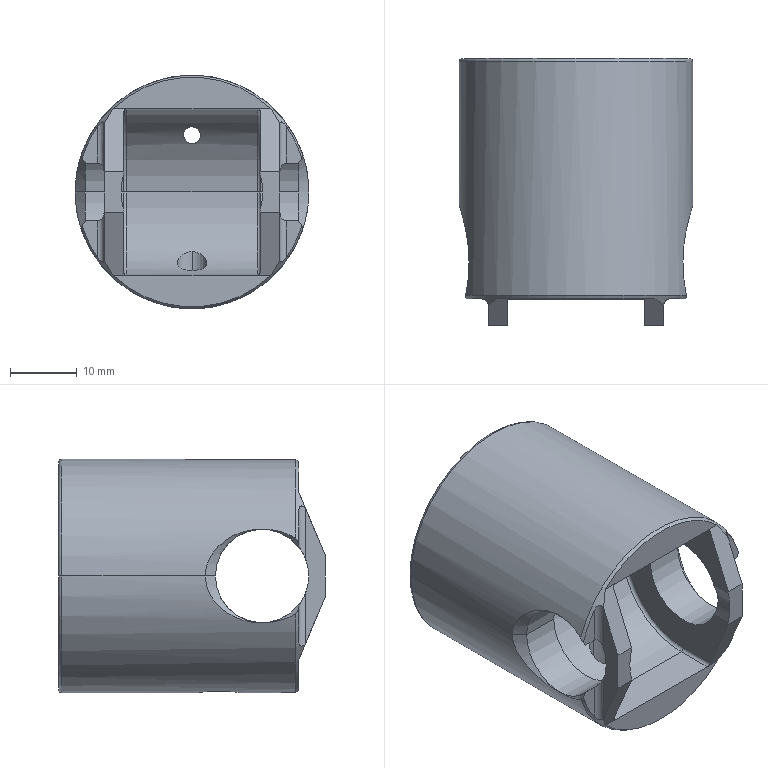Part | SolidWorks | features BaseBody 1 | 1 solid | 78 faces | box 35 x 40 x 35 mm | volume 14028 mm3 | cylinder 29 | plane 22 | cone 14 | torus 12 | spline 1 | commonest cylinder face diameters 1 x4 2 x4 14 x4 21.2 x3 2.5 x2 4.5 x2